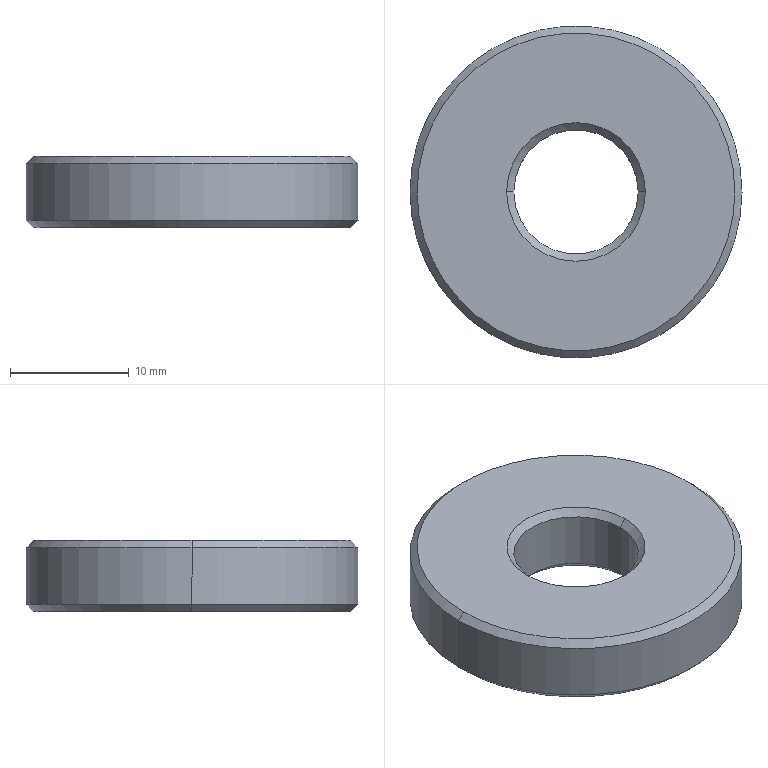Part | SolidWorks | features BaseBody 1 | 1 solid | 38 faces | box 28 x 28 x 6 mm | volume 3096 mm3 | cone 24 | cylinder 12 | plane 2 | commonest cylinder face diameters 2.5 x8 10.5 x2 28 x2
STEP:
#1=CARTESIAN_POINT('',(-5.25,0.,5.4));
#2=VERTEX_POINT('',#1);
#3=CARTESIAN_POINT('',(5.25,0.,5.4));
#4=VERTEX_POINT('',#3);
#5=CARTESIAN_POINT('',(0.,0.,5.4));
#6=DIRECTION('',(0.,0.,1.));
#7=DIRECTION('',(1.,0.,0.));
#8=AXIS2_PLACEMENT_3D('',#5,#6,#7);
#9=CIRCLE('',#8,5.25);
#10=EDGE_CURVE('',#2,#4,#9,.T.);
#11=ORIENTED_EDGE('',*,*,#10,.F.);
#12=CARTESIAN_POINT('',(-5.85,0.,6.));
#13=VERTEX_POINT('',#12);
#14=CARTESIAN_POINT('',(-5.85,0.,6.));
#15=DIRECTION('',(-0.7071,0.,0.7071));
#16=VECTOR('',#15,1000.);
#17=LINE('',#14,#16);
#18=EDGE_CURVE('',#2,#13,#17,.T.);
#19=ORIENTED_EDGE('',*,*,#18,.T.);
#20=CARTESIAN_POINT('',(5.85,0.,6.));
#21=VERTEX_POINT('',#20);
#22=CARTESIAN_POINT('',(0.,0.,6.));
#23=DIRECTION('',(0.,0.,-1.));
#24=DIRECTION('',(1.,0.,0.));
#25=AXIS2_PLACEMENT_3D('',#22,#23,#24);
#26=CIRCLE('',#25,5.85);
#27=EDGE_CURVE('',#21,#13,#26,.T.);
#28=ORIENTED_EDGE('',*,*,#27,.F.);
#29=CARTESIAN_POINT('',(5.85,0.,6.));
#30=DIRECTION('',(0.7071,0.,0.7071));
#31=VECTOR('',#30,1000.);
#32=LINE('',#29,#31);
#33=EDGE_CURVE('',#4,#21,#32,.T.);
#34=ORIENTED_EDGE('',*,*,#33,.F.);
#35=EDGE_LOOP('',(#11,#19,#28,#34));
#36=FACE_OUTER_BOUND('',#35,.T.);
#37=CARTESIAN_POINT('',(0.,0.,6.));
#38=DIRECTION('',(0.,0.,1.));
#39=DIRECTION('',(1.,0.,0.));
#40=AXIS2_PLACEMENT_3D('',#37,#38,#39);
#41=CONICAL_SURFACE('',#40,5.85,0.7854);
#42=ADVANCED_FACE('',(#36),#41,.F.);
#43=CARTESIAN_POINT('',(13.4,0.,6.));
#44=VERTEX_POINT('',#43);
#45=CARTESIAN_POINT('',(-13.4,0.,6.));
#46=VERTEX_POINT('',#45);
#47=CARTESIAN_POINT('',(0.,0.,6.));
#48=DIRECTION('',(0.,0.,1.));
#49=DIRECTION('',(-1.,0.,0.));
#50=AXIS2_PLACEMENT_3D('',#47,#48,#49);
#51=CIRCLE('',#50,13.4);
#52=EDGE_CURVE('',#44,#46,#51,.T.);
#53=ORIENTED_EDGE('',*,*,#52,.F.);
#54=CARTESIAN_POINT('',(14.,0.,5.4));
#55=VERTEX_POINT('',#54);
#56=CARTESIAN_POINT('',(14.,0.,5.4));
#57=DIRECTION('',(0.7071,0.,-0.7071));
#58=VECTOR('',#57,1000.);
#59=LINE('',#56,#58);
#60=EDGE_CURVE('',#44,#55,#59,.T.);
#61=ORIENTED_EDGE('',*,*,#60,.T.);
#62=CARTESIAN_POINT('',(-14.,0.,5.4));
#63=VERTEX_POINT('',#62);
#64=CARTESIAN_POINT('',(0.,0.,5.4));
#65=DIRECTION('',(0.,0.,1.));
#66=DIRECTION('',(-1.,0.,0.));
#67=AXIS2_PLACEMENT_3D('',#64,#65,#66);
#68=CIRCLE('',#67,14.);
#69=EDGE_CURVE('',#55,#63,#68,.T.);
#70=ORIENTED_EDGE('',*,*,#69,.T.);
#71=CARTESIAN_POINT('',(-14.,0.,5.4));
#72=DIRECTION('',(-0.7071,0.,-0.7071));
#73=VECTOR('',#72,1000.);
#74=LINE('',#71,#73);
#75=EDGE_CURVE('',#46,#63,#74,.T.);
#76=ORIENTED_EDGE('',*,*,#75,.F.);
#77=EDGE_LOOP('',(#53,#61,#70,#76));
#78=FACE_OUTER_BOUND('',#77,.T.);
#79=CARTESIAN_POINT('',(0.,0.,5.4));
#80=DIRECTION('',(0.,0.,-1.));
#81=DIRECTION('',(-1.,0.,0.));
#82=AXIS2_PLACEMENT_3D('',#79,#80,#81);
#83=CONICAL_SURFACE('',#82,14.,0.7854);
#84=ADVANCED_FACE('',(#78),#83,.T.);
#85=ORIENTED_EDGE('',*,*,#10,.T.);
#86=CARTESIAN_POINT('',(5.25,0.,0.6));
#87=VERTEX_POINT('',#86);
#88=CARTESIAN_POINT('',(5.25,0.,6.));
#89=DIRECTION('',(0.,0.,-1.));
#90=VECTOR('',#89,1000.);
#91=LINE('',#88,#90);
#92=EDGE_CURVE('',#4,#87,#91,.T.);
#93=ORIENTED_EDGE('',*,*,#92,.T.);
#94=CARTESIAN_POINT('',(-5.25,0.,0.6));
#95=VERTEX_POINT('',#94);
#96=CARTESIAN_POINT('',(0.,0.,0.6));
#97=DIRECTION('',(0.,0.,1.));
#98=DIRECTION('',(-1.,0.,0.));
#99=AXIS2_PLACEMENT_3D('',#96,#97,#98);
#100=CIRCLE('',#99,5.25);
#101=EDGE_CURVE('',#95,#87,#100,.T.);
#102=ORIENTED_EDGE('',*,*,#101,.F.);
#103=CARTESIAN_POINT('',(-5.25,0.,6.));
#104=DIRECTION('',(0.,0.,-1.));
#105=VECTOR('',#104,1000.);
#106=LINE('',#103,#105);
#107=EDGE_CURVE('',#2,#95,#106,.T.);
#108=ORIENTED_EDGE('',*,*,#107,.F.);
#109=EDGE_LOOP('',(#85,#93,#102,#108));
#110=FACE_OUTER_BOUND('',#109,.T.);
#111=CARTESIAN_POINT('',(0.,0.,6.));
#112=DIRECTION('',(0.,0.,-1.));
#113=DIRECTION('',(-1.,0.,0.));
#114=AXIS2_PLACEMENT_3D('',#111,#112,#113);
#115=CYLINDRICAL_SURFACE('',#114,5.25);
#116=ADVANCED_FACE('',(#110),#115,.F.);
#117=ORIENTED_EDGE('',*,*,#69,.F.);
#118=CARTESIAN_POINT('',(14.,0.,0.6));
#119=VERTEX_POINT('',#118);
#120=CARTESIAN_POINT('',(14.,0.,6.));
#121=DIRECTION('',(0.,0.,-1.));
#122=VECTOR('',#121,1000.);
#123=LINE('',#120,#122);
#124=EDGE_CURVE('',#55,#119,#123,.T.);
#125=ORIENTED_EDGE('',*,*,#124,.T.);
#126=CARTESIAN_POINT('',(-14.,0.,0.6));
#127=VERTEX_POINT('',#126);
#128=CARTESIAN_POINT('',(0.,0.,0.6));
#129=DIRECTION('',(0.,0.,1.));
#130=DIRECTION('',(-1.,0.,0.));
#131=AXIS2_PLACEMENT_3D('',#128,#129,#130);
#132=CIRCLE('',#131,14.);
#133=EDGE_CURVE('',#119,#127,#132,.T.);
#134=ORIENTED_EDGE('',*,*,#133,.T.);
#135=CARTESIAN_POINT('',(-14.,0.,6.));
#136=DIRECTION('',(0.,0.,-1.));
#137=VECTOR('',#136,1000.);
#138=LINE('',#135,#137);
#139=EDGE_CURVE('',#63,#127,#138,.T.);
#140=ORIENTED_EDGE('',*,*,#139,.F.);
#141=EDGE_LOOP('',(#117,#125,#134,#140));
#142=FACE_OUTER_BOUND('',#141,.T.);
#143=CARTESIAN_POINT('',(0.,0.,6.));
#144=DIRECTION('',(0.,0.,-1.));
#145=DIRECTION('',(-1.,0.,0.));
#146=AXIS2_PLACEMENT_3D('',#143,#144,#145);
#147=CYLINDRICAL_SURFACE('',#146,14.);
#148=ADVANCED_FACE('',(#142),#147,.T.);
#149=ORIENTED_EDGE('',*,*,#101,.T.);
#150=CARTESIAN_POINT('',(5.85,0.,0.));
#151=VERTEX_POINT('',#150);
#152=CARTESIAN_POINT('',(5.85,0.,0.));
#153=DIRECTION('',(0.7071,0.,-0.7071));
#154=VECTOR('',#153,1000.);
#155=LINE('',#152,#154);
#156=EDGE_CURVE('',#87,#151,#155,.T.);
#157=ORIENTED_EDGE('',*,*,#156,.T.);
#158=CARTESIAN_POINT('',(-5.85,0.,0.));
#159=VERTEX_POINT('',#158);
#160=CARTESIAN_POINT('',(0.,0.,0.));
#161=DIRECTION('',(0.,0.,1.));
#162=DIRECTION('',(-1.,0.,0.));
#163=AXIS2_PLACEMENT_3D('',#160,#161,#162);
#164=CIRCLE('',#163,5.85);
#165=EDGE_CURVE('',#159,#151,#164,.T.);
#166=ORIENTED_EDGE('',*,*,#165,.F.);
#167=CARTESIAN_POINT('',(-5.85,0.,0.));
#168=DIRECTION('',(-0.7071,0.,-0.7071));
#169=VECTOR('',#168,1000.);
#170=LINE('',#167,#169);
#171=EDGE_CURVE('',#95,#159,#170,.T.);
#172=ORIENTED_EDGE('',*,*,#171,.F.);
#173=EDGE_LOOP('',(#149,#157,#166,#172));
#174=FACE_OUTER_BOUND('',#173,.T.);
#175=CARTESIAN_POINT('',(0.,0.,0.));
#176=DIRECTION('',(0.,0.,-1.));
#177=DIRECTION('',(-1.,0.,0.));
#178=AXIS2_PLACEMENT_3D('',#175,#176,#177);
#179=CONICAL_SURFACE('',#178,5.85,0.7854);
#180=ADVANCED_FACE('',(#174),#179,.F.);
#181=CARTESIAN_POINT('',(13.4,0.,0.));
#182=VERTEX_POINT('',#181);
#183=CARTESIAN_POINT('',(-13.4,0.,0.));
#184=VERTEX_POINT('',#183);
#185=CARTESIAN_POINT('',(0.,0.,0.));
#186=DIRECTION('',(0.,0.,1.));
#187=DIRECTION('',(1.,0.,0.));
#188=AXIS2_PLACEMENT_3D('',#185,#186,#187);
#189=CIRCLE('',#188,13.4);
#190=EDGE_CURVE('',#182,#184,#189,.T.);
#191=ORIENTED_EDGE('',*,*,#190,.T.);
#192=CARTESIAN_POINT('',(-14.,0.,0.6));
#193=DIRECTION('',(-0.7071,0.,0.7071));
#194=VECTOR('',#193,1000.);
#195=LINE('',#192,#194);
#196=EDGE_CURVE('',#184,#127,#195,.T.);
#197=ORIENTED_EDGE('',*,*,#196,.T.);
#198=ORIENTED_EDGE('',*,*,#133,.F.);
#199=CARTESIAN_POINT('',(14.,0.,0.6));
#200=DIRECTION('',(0.7071,0.,0.7071));
#201=VECTOR('',#200,1000.);
#202=LINE('',#199,#201);
#203=EDGE_CURVE('',#182,#119,#202,.T.);
#204=ORIENTED_EDGE('',*,*,#203,.F.);
#205=EDGE_LOOP('',(#191,#197,#198,#204));
#206=FACE_OUTER_BOUND('',#205,.T.);
#207=CARTESIAN_POINT('',(0.,0.,0.6));
#208=DIRECTION('',(0.,0.,1.));
#209=DIRECTION('',(1.,0.,0.));
#210=AXIS2_PLACEMENT_3D('',#207,#208,#209);
#211=CONICAL_SURFACE('',#210,14.,0.7854);
#212=ADVANCED_FACE('',(#206),#211,.T.);
#213=CARTESIAN_POINT('',(1.25,9.5,0.4));
#214=VERTEX_POINT('',#213);
#215=CARTESIAN_POINT('',(-1.25,9.5,0.4));
#216=VERTEX_POINT('',#215);
#217=CARTESIAN_POINT('',(0.,9.5,0.4));
#218=DIRECTION('',(0.,0.,-1.));
#219=DIRECTION('',(1.,0.,0.));
#220=AXIS2_PLACEMENT_3D('',#217,#218,#219);
#221=CIRCLE('',#220,1.25);
#222=EDGE_CURVE('',#214,#216,#221,.T.);
#223=ORIENTED_EDGE('',*,*,#222,.F.);
#224=CARTESIAN_POINT('',(1.65,9.5,0.));
#225=VERTEX_POINT('',#224);
#226=CARTESIAN_POINT('',(1.65,9.5,0.));
#227=DIRECTION('',(0.7071,0.,-0.7071));
#228=VECTOR('',#227,1000.);
#229=LINE('',#226,#228);
#230=EDGE_CURVE('',#214,#225,#229,.T.);
#231=ORIENTED_EDGE('',*,*,#230,.T.);
#232=CARTESIAN_POINT('',(-1.65,9.5,0.));
#233=VERTEX_POINT('',#232);
#234=CARTESIAN_POINT('',(0.,9.5,0.));
#235=DIRECTION('',(0.,0.,-1.));
#236=DIRECTION('',(-1.,0.,0.));
#237=AXIS2_PLACEMENT_3D('',#234,#235,#236);
#238=CIRCLE('',#237,1.65);
#239=EDGE_CURVE('',#225,#233,#238,.T.);
#240=ORIENTED_EDGE('',*,*,#239,.T.);
#241=CARTESIAN_POINT('',(-1.65,9.5,0.));
#242=DIRECTION('',(-0.7071,0.,-0.7071));
#243=VECTOR('',#242,1000.);
#244=LINE('',#241,#243);
#245=EDGE_CURVE('',#216,#233,#244,.T.);
#246=ORIENTED_EDGE('',*,*,#245,.F.);
#247=EDGE_LOOP('',(#223,#231,#240,#246));
#248=FACE_OUTER_BOUND('',#247,.T.);
#249=CARTESIAN_POINT('',(0.,9.5,0.));
#250=DIRECTION('',(0.,0.,-1.));
#251=DIRECTION('',(-1.,0.,0.));
#252=AXIS2_PLACEMENT_3D('',#249,#250,#251);
#253=CONICAL_SURFACE('',#252,1.65,0.7854);
#254=ADVANCED_FACE('',(#248),#253,.F.);
#255=CARTESIAN_POINT('',(10.75,0.,0.4));
#256=VERTEX_POINT('',#255);
#257=CARTESIAN_POINT('',(8.25,0.,0.4));
#258=VERTEX_POINT('',#257);
#259=CARTESIAN_POINT('',(9.5,0.,0.4));
#260=DIRECTION('',(0.,0.,-1.));
#261=DIRECTION('',(1.,0.,0.));
#262=AXIS2_PLACEMENT_3D('',#259,#260,#261);
#263=CIRCLE('',#262,1.25);
#264=EDGE_CURVE('',#256,#258,#263,.T.);
#265=ORIENTED_EDGE('',*,*,#264,.F.);
#266=CARTESIAN_POINT('',(11.15,0.,0.));
#267=VERTEX_POINT('',#266);
#268=CARTESIAN_POINT('',(11.15,0.,0.));
#269=DIRECTION('',(0.7071,0.,-0.7071));
#270=VECTOR('',#269,1000.);
#271=LINE('',#268,#270);
#272=EDGE_CURVE('',#256,#267,#271,.T.);
#273=ORIENTED_EDGE('',*,*,#272,.T.);
#274=CARTESIAN_POINT('',(7.85,0.,0.));
#275=VERTEX_POINT('',#274);
#276=CARTESIAN_POINT('',(9.5,0.,0.));
#277=DIRECTION('',(0.,0.,-1.));
#278=DIRECTION('',(-1.,0.,0.));
#279=AXIS2_PLACEMENT_3D('',#276,#277,#278);
#280=CIRCLE('',#279,1.65);
#281=EDGE_CURVE('',#267,#275,#280,.T.);
#282=ORIENTED_EDGE('',*,*,#281,.T.);
#283=CARTESIAN_POINT('',(7.85,0.,0.));
#284=DIRECTION('',(-0.7071,0.,-0.7071));
#285=VECTOR('',#284,1000.);
#286=LINE('',#283,#285);
#287=EDGE_CURVE('',#258,#275,#286,.T.);
#288=ORIENTED_EDGE('',*,*,#287,.F.);
#289=EDGE_LOOP('',(#265,#273,#282,#288));
#290=FACE_OUTER_BOUND('',#289,.T.);
#291=CARTESIAN_POINT('',(9.5,0.,0.));
#292=DIRECTION('',(0.,0.,-1.));
#293=DIRECTION('',(-1.,0.,0.));
#294=AXIS2_PLACEMENT_3D('',#291,#292,#293);
#295=CONICAL_SURFACE('',#294,1.65,0.7854);
#296=ADVANCED_FACE('',(#290),#295,.F.);
#297=CARTESIAN_POINT('',(1.25,-9.5,0.4));
#298=VERTEX_POINT('',#297);
#299=CARTESIAN_POINT('',(-1.25,-9.5,0.4));
#300=VERTEX_POINT('',#299);
#301=CARTESIAN_POINT('',(0.,-9.5,0.4));
#302=DIRECTION('',(0.,0.,-1.));
#303=DIRECTION('',(1.,0.,0.));
#304=AXIS2_PLACEMENT_3D('',#301,#302,#303);
#305=CIRCLE('',#304,1.25);
#306=EDGE_CURVE('',#298,#300,#305,.T.);
#307=ORIENTED_EDGE('',*,*,#306,.F.);
#308=CARTESIAN_POINT('',(1.65,-9.5,0.));
#309=VERTEX_POINT('',#308);
#310=CARTESIAN_POINT('',(1.65,-9.5,0.));
#311=DIRECTION('',(0.7071,0.,-0.7071));
#312=VECTOR('',#311,1000.);
#313=LINE('',#310,#312);
#314=EDGE_CURVE('',#298,#309,#313,.T.);
#315=ORIENTED_EDGE('',*,*,#314,.T.);
#316=CARTESIAN_POINT('',(-1.65,-9.5,0.));
#317=VERTEX_POINT('',#316);
#318=CARTESIAN_POINT('',(0.,-9.5,0.));
#319=DIRECTION('',(0.,0.,-1.));
#320=DIRECTION('',(-1.,0.,0.));
#321=AXIS2_PLACEMENT_3D('',#318,#319,#320);
#322=CIRCLE('',#321,1.65);
#323=EDGE_CURVE('',#309,#317,#322,.T.);
#324=ORIENTED_EDGE('',*,*,#323,.T.);
#325=CARTESIAN_POINT('',(-1.65,-9.5,0.));
#326=DIRECTION('',(-0.7071,0.,-0.7071));
#327=VECTOR('',#326,1000.);
#328=LINE('',#325,#327);
#329=EDGE_CURVE('',#300,#317,#328,.T.);
#330=ORIENTED_EDGE('',*,*,#329,.F.);
#331=EDGE_LOOP('',(#307,#315,#324,#330));
#332=FACE_OUTER_BOUND('',#331,.T.);
#333=CARTESIAN_POINT('',(0.,-9.5,0.));
#334=DIRECTION('',(0.,0.,-1.));
#335=DIRECTION('',(-1.,0.,0.));
#336=AXIS2_PLACEMENT_3D('',#333,#334,#335);
#337=CONICAL_SURFACE('',#336,1.65,0.7854);
#338=ADVANCED_FACE('',(#332),#337,.F.);
#339=CARTESIAN_POINT('',(-8.25,0.,0.4));
#340=VERTEX_POINT('',#339);
#341=CARTESIAN_POINT('',(-10.75,0.,0.4));
#342=VERTEX_POINT('',#341);
#343=CARTESIAN_POINT('',(-9.5,0.,0.4));
#344=DIRECTION('',(0.,0.,-1.));
#345=DIRECTION('',(1.,0.,0.));
#346=AXIS2_PLACEMENT_3D('',#343,#344,#345);
#347=CIRCLE('',#346,1.25);
#348=EDGE_CURVE('',#340,#342,#347,.T.);
#349=ORIENTED_EDGE('',*,*,#348,.F.);
#350=CARTESIAN_POINT('',(-7.85,0.,0.));
#351=VERTEX_POINT('',#350);
#352=CARTESIAN_POINT('',(-7.85,0.,0.));
#353=DIRECTION('',(0.7071,0.,-0.7071));
#354=VECTOR('',#353,1000.);
#355=LINE('',#352,#354);
#356=EDGE_CURVE('',#340,#351,#355,.T.);
#357=ORIENTED_EDGE('',*,*,#356,.T.);
#358=CARTESIAN_POINT('',(-11.15,0.,0.));
#359=VERTEX_POINT('',#358);
#360=CARTESIAN_POINT('',(-9.5,0.,0.));
#361=DIRECTION('',(0.,0.,-1.));
#362=DIRECTION('',(-1.,0.,0.));
#363=AXIS2_PLACEMENT_3D('',#360,#361,#362);
#364=CIRCLE('',#363,1.65);
#365=EDGE_CURVE('',#351,#359,#364,.T.);
#366=ORIENTED_EDGE('',*,*,#365,.T.);
#367=CARTESIAN_POINT('',(-11.15,0.,0.));
#368=DIRECTION('',(-0.7071,0.,-0.7071));
#369=VECTOR('',#368,1000.);
#370=LINE('',#367,#369);
#371=EDGE_CURVE('',#342,#359,#370,.T.);
#372=ORIENTED_EDGE('',*,*,#371,.F.);
#373=EDGE_LOOP('',(#349,#357,#366,#372));
#374=FACE_OUTER_BOUND('',#373,.T.);
#375=CARTESIAN_POINT('',(-9.5,0.,0.));
#376=DIRECTION('',(0.,0.,-1.));
#377=DIRECTION('',(-1.,0.,0.));
#378=AXIS2_PLACEMENT_3D('',#375,#376,#377);
#379=CONICAL_SURFACE('',#378,1.65,0.7854);
#380=ADVANCED_FACE('',(#374),#379,.F.);
#381=ORIENTED_EDGE('',*,*,#222,.T.);
#382=CARTESIAN_POINT('',(-1.25,9.5,1.25));
#383=VERTEX_POINT('',#382);
#384=CARTESIAN_POINT('',(-1.25,9.5,2.5));
#385=DIRECTION('',(0.,0.,1.));
#386=VECTOR('',#385,1000.);
#387=LINE('',#384,#386);
#388=EDGE_CURVE('',#216,#383,#387,.T.);
#389=ORIENTED_EDGE('',*,*,#388,.T.);
#390=CARTESIAN_POINT('',(1.25,9.5,1.25));
#391=VERTEX_POINT('',#390);
#392=CARTESIAN_POINT('',(0.,9.5,1.25));
#393=DIRECTION('',(0.,0.,-1.));
#394=DIRECTION('',(1.,0.,0.));
#395=AXIS2_PLACEMENT_3D('',#392,#393,#394);
#396=CIRCLE('',#395,1.25);
#397=EDGE_CURVE('',#391,#383,#396,.T.);
#398=ORIENTED_EDGE('',*,*,#397,.F.);
#399=CARTESIAN_POINT('',(1.25,9.5,2.5));
#400=DIRECTION('',(0.,0.,1.));
#401=VECTOR('',#400,1000.);
#402=LINE('',#399,#401);
#403=EDGE_CURVE('',#214,#391,#402,.T.);
#404=ORIENTED_EDGE('',*,*,#403,.F.);
#405=EDGE_LOOP('',(#381,#389,#398,#404));
#406=FACE_OUTER_BOUND('',#405,.T.);
#407=CARTESIAN_POINT('',(0.,9.5,2.5));
#408=DIRECTION('',(0.,0.,1.));
#409=DIRECTION('',(1.,0.,0.));
#410=AXIS2_PLACEMENT_3D('',#407,#408,#409);
#411=CYLINDRICAL_SURFACE('',#410,1.25);
#412=ADVANCED_FACE('',(#406),#411,.F.);
#413=ORIENTED_EDGE('',*,*,#264,.T.);
#414=CARTESIAN_POINT('',(8.25,0.,1.25));
#415=VERTEX_POINT('',#414);
#416=CARTESIAN_POINT('',(8.25,0.,2.5));
#417=DIRECTION('',(0.,0.,1.));
#418=VECTOR('',#417,1000.);
#419=LINE('',#416,#418);
#420=EDGE_CURVE('',#258,#415,#419,.T.);
#421=ORIENTED_EDGE('',*,*,#420,.T.);
#422=CARTESIAN_POINT('',(10.75,0.,1.25));
#423=VERTEX_POINT('',#422);
#424=CARTESIAN_POINT('',(9.5,0.,1.25));
#425=DIRECTION('',(0.,0.,-1.));
#426=DIRECTION('',(1.,0.,0.));
#427=AXIS2_PLACEMENT_3D('',#424,#425,#426);
#428=CIRCLE('',#427,1.25);
#429=EDGE_CURVE('',#423,#415,#428,.T.);
#430=ORIENTED_EDGE('',*,*,#429,.F.);
#431=CARTESIAN_POINT('',(10.75,0.,2.5));
#432=DIRECTION('',(0.,0.,1.));
#433=VECTOR('',#432,1000.);
#434=LINE('',#431,#433);
#435=EDGE_CURVE('',#256,#423,#434,.T.);
#436=ORIENTED_EDGE('',*,*,#435,.F.);
#437=EDGE_LOOP('',(#413,#421,#430,#436));
#438=FACE_OUTER_BOUND('',#437,.T.);
#439=CARTESIAN_POINT('',(9.5,0.,2.5));
#440=DIRECTION('',(0.,0.,1.));
#441=DIRECTION('',(1.,0.,0.));
#442=AXIS2_PLACEMENT_3D('',#439,#440,#441);
#443=CYLINDRICAL_SURFACE('',#442,1.25);
#444=ADVANCED_FACE('',(#438),#443,.F.);
#445=ORIENTED_EDGE('',*,*,#306,.T.);
#446=CARTESIAN_POINT('',(-1.25,-9.5,1.25));
#447=VERTEX_POINT('',#446);
#448=CARTESIAN_POINT('',(-1.25,-9.5,2.5));
#449=DIRECTION('',(0.,0.,1.));
#450=VECTOR('',#449,1000.);
#451=LINE('',#448,#450);
#452=EDGE_CURVE('',#300,#447,#451,.T.);
#453=ORIENTED_EDGE('',*,*,#452,.T.);
#454=CARTESIAN_POINT('',(1.25,-9.5,1.25));
#455=VERTEX_POINT('',#454);
#456=CARTESIAN_POINT('',(0.,-9.5,1.25));
#457=DIRECTION('',(0.,0.,-1.));
#458=DIRECTION('',(1.,0.,0.));
#459=AXIS2_PLACEMENT_3D('',#456,#457,#458);
#460=CIRCLE('',#459,1.25);
#461=EDGE_CURVE('',#455,#447,#460,.T.);
#462=ORIENTED_EDGE('',*,*,#461,.F.);
#463=CARTESIAN_POINT('',(1.25,-9.5,2.5));
#464=DIRECTION('',(0.,0.,1.));
#465=VECTOR('',#464,1000.);
#466=LINE('',#463,#465);
#467=EDGE_CURVE('',#298,#455,#466,.T.);
#468=ORIENTED_EDGE('',*,*,#467,.F.);
#469=EDGE_LOOP('',(#445,#453,#462,#468));
#470=FACE_OUTER_BOUND('',#469,.T.);
#471=CARTESIAN_POINT('',(0.,-9.5,2.5));
#472=DIRECTION('',(0.,0.,1.));
#473=DIRECTION('',(1.,0.,0.));
#474=AXIS2_PLACEMENT_3D('',#471,#472,#473);
#475=CYLINDRICAL_SURFACE('',#474,1.25);
#476=ADVANCED_FACE('',(#470),#475,.F.);
#477=ORIENTED_EDGE('',*,*,#348,.T.);
#478=CARTESIAN_POINT('',(-10.75,0.,1.25));
#479=VERTEX_POINT('',#478);
#480=CARTESIAN_POINT('',(-10.75,0.,2.5));
#481=DIRECTION('',(0.,0.,1.));
#482=VECTOR('',#481,1000.);
#483=LINE('',#480,#482);
#484=EDGE_CURVE('',#342,#479,#483,.T.);
#485=ORIENTED_EDGE('',*,*,#484,.T.);
#486=CARTESIAN_POINT('',(-8.25,0.,1.25));
#487=VERTEX_POINT('',#486);
#488=CARTESIAN_POINT('',(-9.5,0.,1.25));
#489=DIRECTION('',(0.,0.,-1.));
#490=DIRECTION('',(1.,0.,0.));
#491=AXIS2_PLACEMENT_3D('',#488,#489,#490);
#492=CIRCLE('',#491,1.25);
#493=EDGE_CURVE('',#487,#479,#492,.T.);
#494=ORIENTED_EDGE('',*,*,#493,.F.);
#495=CARTESIAN_POINT('',(-8.25,0.,2.5));
#496=DIRECTION('',(0.,0.,1.));
#497=VECTOR('',#496,1000.);
#498=LINE('',#495,#497);
#499=EDGE_CURVE('',#340,#487,#498,.T.);
#500=ORIENTED_EDGE('',*,*,#499,.F.);
#501=EDGE_LOOP('',(#477,#485,#494,#500));
#502=FACE_OUTER_BOUND('',#501,.T.);
#503=CARTESIAN_POINT('',(-9.5,0.,2.5));
#504=DIRECTION('',(0.,0.,1.));
#505=DIRECTION('',(1.,0.,0.));
#506=AXIS2_PLACEMENT_3D('',#503,#504,#505);
#507=CYLINDRICAL_SURFACE('',#506,1.25);
#508=ADVANCED_FACE('',(#502),#507,.F.);
#509=CARTESIAN_POINT('',(0.,9.5,2.5));
#510=VERTEX_POINT('',#509);
#511=CARTESIAN_POINT('',(-1.25,9.5,1.25));
#512=DIRECTION('',(-0.7071,0.,-0.7071));
#513=VECTOR('',#512,1000.);
#514=LINE('',#511,#513);
#515=EDGE_CURVE('',#510,#383,#514,.T.);
#516=ORIENTED_EDGE('',*,*,#515,.F.);
#517=CARTESIAN_POINT('',(1.25,9.5,1.25));
#518=DIRECTION('',(0.7071,0.,-0.7071));
#519=VECTOR('',#518,1000.);
#520=LINE('',#517,#519);
#521=EDGE_CURVE('',#510,#391,#520,.T.);
#522=ORIENTED_EDGE('',*,*,#521,.T.);
#523=ORIENTED_EDGE('',*,*,#397,.T.);
#524=EDGE_LOOP('',(#516,#522,#523));
#525=FACE_OUTER_BOUND('',#524,.T.);
#526=CARTESIAN_POINT('',(0.,9.5,1.25));
#527=DIRECTION('',(0.,0.,-1.));
#528=DIRECTION('',(-1.,0.,0.));
#529=AXIS2_PLACEMENT_3D('',#526,#527,#528);
#530=CONICAL_SURFACE('',#529,1.25,0.7854);
#531=ADVANCED_FACE('',(#525),#530,.F.);
#532=CARTESIAN_POINT('',(9.5,0.,2.5));
#533=VERTEX_POINT('',#532);
#534=CARTESIAN_POINT('',(8.25,0.,1.25));
#535=DIRECTION('',(-0.7071,0.,-0.7071));
#536=VECTOR('',#535,1000.);
#537=LINE('',#534,#536);
#538=EDGE_CURVE('',#533,#415,#537,.T.);
#539=ORIENTED_EDGE('',*,*,#538,.F.);
#540=CARTESIAN_POINT('',(10.75,0.,1.25));
#541=DIRECTION('',(0.7071,0.,-0.7071));
#542=VECTOR('',#541,1000.);
#543=LINE('',#540,#542);
#544=EDGE_CURVE('',#533,#423,#543,.T.);
#545=ORIENTED_EDGE('',*,*,#544,.T.);
#546=ORIENTED_EDGE('',*,*,#429,.T.);
#547=EDGE_LOOP('',(#539,#545,#546));
#548=FACE_OUTER_BOUND('',#547,.T.);
#549=CARTESIAN_POINT('',(9.5,0.,1.25));
#550=DIRECTION('',(0.,0.,-1.));
#551=DIRECTION('',(-1.,0.,0.));
#552=AXIS2_PLACEMENT_3D('',#549,#550,#551);
#553=CONICAL_SURFACE('',#552,1.25,0.7854);
#554=ADVANCED_FACE('',(#548),#553,.F.);
#555=CARTESIAN_POINT('',(0.,-9.5,2.5));
#556=VERTEX_POINT('',#555);
#557=CARTESIAN_POINT('',(-1.25,-9.5,1.25));
#558=DIRECTION('',(-0.7071,0.,-0.7071));
#559=VECTOR('',#558,1000.);
#560=LINE('',#557,#559);
#561=EDGE_CURVE('',#556,#447,#560,.T.);
#562=ORIENTED_EDGE('',*,*,#561,.F.);
#563=CARTESIAN_POINT('',(1.25,-9.5,1.25));
#564=DIRECTION('',(0.7071,0.,-0.7071));
#565=VECTOR('',#564,1000.);
#566=LINE('',#563,#565);
#567=EDGE_CURVE('',#556,#455,#566,.T.);
#568=ORIENTED_EDGE('',*,*,#567,.T.);
#569=ORIENTED_EDGE('',*,*,#461,.T.);
#570=EDGE_LOOP('',(#562,#568,#569));
#571=FACE_OUTER_BOUND('',#570,.T.);
#572=CARTESIAN_POINT('',(0.,-9.5,1.25));
#573=DIRECTION('',(0.,0.,-1.));
#574=DIRECTION('',(-1.,0.,0.));
#575=AXIS2_PLACEMENT_3D('',#572,#573,#574);
#576=CONICAL_SURFACE('',#575,1.25,0.7854);
#577=ADVANCED_FACE('',(#571),#576,.F.);
#578=CARTESIAN_POINT('',(-9.5,0.,2.5));
#579=VERTEX_POINT('',#578);
#580=CARTESIAN_POINT('',(-10.75,0.,1.25));
#581=DIRECTION('',(-0.7071,0.,-0.7071));
#582=VECTOR('',#581,1000.);
#583=LINE('',#580,#582);
#584=EDGE_CURVE('',#579,#479,#583,.T.);
#585=ORIENTED_EDGE('',*,*,#584,.F.);
#586=CARTESIAN_POINT('',(-8.25,0.,1.25));
#587=DIRECTION('',(0.7071,0.,-0.7071));
#588=VECTOR('',#587,1000.);
#589=LINE('',#586,#588);
#590=EDGE_CURVE('',#579,#487,#589,.T.);
#591=ORIENTED_EDGE('',*,*,#590,.T.);
#592=ORIENTED_EDGE('',*,*,#493,.T.);
#593=EDGE_LOOP('',(#585,#591,#592));
#594=FACE_OUTER_BOUND('',#593,.T.);
#595=CARTESIAN_POINT('',(-9.5,0.,1.25));
#596=DIRECTION('',(0.,0.,-1.));
#597=DIRECTION('',(-1.,0.,0.));
#598=AXIS2_PLACEMENT_3D('',#595,#596,#597);
#599=CONICAL_SURFACE('',#598,1.25,0.7854);
#600=ADVANCED_FACE('',(#594),#599,.F.);
#601=ORIENTED_EDGE('',*,*,#27,.T.);
#602=CARTESIAN_POINT('',(0.,0.,6.));
#603=DIRECTION('',(0.,0.,-1.));
#604=DIRECTION('',(1.,0.,0.));
#605=AXIS2_PLACEMENT_3D('',#602,#603,#604);
#606=CIRCLE('',#605,5.85);
#607=EDGE_CURVE('',#13,#21,#606,.T.);
#608=ORIENTED_EDGE('',*,*,#607,.T.);
#609=EDGE_LOOP('',(#601,#608));
#610=FACE_BOUND('',#609,.T.);
#611=CARTESIAN_POINT('',(0.,0.,6.));
#612=DIRECTION('',(0.,0.,1.));
#613=DIRECTION('',(-1.,0.,0.));
#614=AXIS2_PLACEMENT_3D('',#611,#612,#613);
#615=CIRCLE('',#614,13.4);
#616=EDGE_CURVE('',#46,#44,#615,.T.);
#617=ORIENTED_EDGE('',*,*,#616,.T.);
#618=ORIENTED_EDGE('',*,*,#52,.T.);
#619=EDGE_LOOP('',(#617,#618));
#620=FACE_OUTER_BOUND('',#619,.T.);
#621=CARTESIAN_POINT('',(0.,0.,6.));
#622=DIRECTION('',(0.,0.,1.));
#623=DIRECTION('',(1.,0.,0.));
#624=AXIS2_PLACEMENT_3D('',#621,#622,#623);
#625=PLANE('',#624);
#626=ADVANCED_FACE('',(#610,#620),#625,.T.);
#627=ORIENTED_EDGE('',*,*,#18,.F.);
#628=CARTESIAN_POINT('',(0.,0.,5.4));
#629=DIRECTION('',(0.,0.,1.));
#630=DIRECTION('',(1.,0.,0.));
#631=AXIS2_PLACEMENT_3D('',#628,#629,#630);
#632=CIRCLE('',#631,5.25);
#633=EDGE_CURVE('',#4,#2,#632,.T.);
#634=ORIENTED_EDGE('',*,*,#633,.F.);
#635=ORIENTED_EDGE('',*,*,#33,.T.);
#636=ORIENTED_EDGE('',*,*,#607,.F.);
#637=EDGE_LOOP('',(#627,#634,#635,#636));
#638=FACE_OUTER_BOUND('',#637,.T.);
#639=CARTESIAN_POINT('',(0.,0.,6.));
#640=DIRECTION('',(0.,0.,1.));
#641=DIRECTION('',(1.,0.,0.));
#642=AXIS2_PLACEMENT_3D('',#639,#640,#641);
#643=CONICAL_SURFACE('',#642,5.85,0.7854);
#644=ADVANCED_FACE('',(#638),#643,.F.);
#645=ORIENTED_EDGE('',*,*,#60,.F.);
#646=ORIENTED_EDGE('',*,*,#616,.F.);
#647=ORIENTED_EDGE('',*,*,#75,.T.);
#648=CARTESIAN_POINT('',(0.,0.,5.4));
#649=DIRECTION('',(0.,0.,1.));
#650=DIRECTION('',(-1.,0.,0.));
#651=AXIS2_PLACEMENT_3D('',#648,#649,#650);
#652=CIRCLE('',#651,14.);
#653=EDGE_CURVE('',#63,#55,#652,.T.);
#654=ORIENTED_EDGE('',*,*,#653,.T.);
#655=EDGE_LOOP('',(#645,#646,#647,#654));
#656=FACE_OUTER_BOUND('',#655,.T.);
#657=CARTESIAN_POINT('',(0.,0.,5.4));
#658=DIRECTION('',(0.,0.,-1.));
#659=DIRECTION('',(-1.,0.,0.));
#660=AXIS2_PLACEMENT_3D('',#657,#658,#659);
#661=CONICAL_SURFACE('',#660,14.,0.7854);
#662=ADVANCED_FACE('',(#656),#661,.T.);
#663=ORIENTED_EDGE('',*,*,#92,.F.);
#664=ORIENTED_EDGE('',*,*,#633,.T.);
#665=ORIENTED_EDGE('',*,*,#107,.T.);
#666=CARTESIAN_POINT('',(0.,0.,0.6));
#667=DIRECTION('',(0.,0.,1.));
#668=DIRECTION('',(-1.,0.,0.));
#669=AXIS2_PLACEMENT_3D('',#666,#667,#668);
#670=CIRCLE('',#669,5.25);
#671=EDGE_CURVE('',#87,#95,#670,.T.);
#672=ORIENTED_EDGE('',*,*,#671,.F.);
#673=EDGE_LOOP('',(#663,#664,#665,#672));
#674=FACE_OUTER_BOUND('',#673,.T.);
#675=CARTESIAN_POINT('',(0.,0.,6.));
#676=DIRECTION('',(0.,0.,-1.));
#677=DIRECTION('',(-1.,0.,0.));
#678=AXIS2_PLACEMENT_3D('',#675,#676,#677);
#679=CYLINDRICAL_SURFACE('',#678,5.25);
#680=ADVANCED_FACE('',(#674),#679,.F.);
#681=ORIENTED_EDGE('',*,*,#124,.F.);
#682=ORIENTED_EDGE('',*,*,#653,.F.);
#683=ORIENTED_EDGE('',*,*,#139,.T.);
#684=CARTESIAN_POINT('',(0.,0.,0.6));
#685=DIRECTION('',(0.,0.,1.));
#686=DIRECTION('',(-1.,0.,0.));
#687=AXIS2_PLACEMENT_3D('',#684,#685,#686);
#688=CIRCLE('',#687,14.);
#689=EDGE_CURVE('',#127,#119,#688,.T.);
#690=ORIENTED_EDGE('',*,*,#689,.T.);
#691=EDGE_LOOP('',(#681,#682,#683,#690));
#692=FACE_OUTER_BOUND('',#691,.T.);
#693=CARTESIAN_POINT('',(0.,0.,6.));
#694=DIRECTION('',(0.,0.,-1.));
#695=DIRECTION('',(-1.,0.,0.));
#696=AXIS2_PLACEMENT_3D('',#693,#694,#695);
#697=CYLINDRICAL_SURFACE('',#696,14.);
#698=ADVANCED_FACE('',(#692),#697,.T.);
#699=ORIENTED_EDGE('',*,*,#156,.F.);
#700=ORIENTED_EDGE('',*,*,#671,.T.);
#701=ORIENTED_EDGE('',*,*,#171,.T.);
#702=CARTESIAN_POINT('',(0.,0.,0.));
#703=DIRECTION('',(0.,0.,1.));
#704=DIRECTION('',(-1.,0.,0.));
#705=AXIS2_PLACEMENT_3D('',#702,#703,#704);
#706=CIRCLE('',#705,5.85);
#707=EDGE_CURVE('',#151,#159,#706,.T.);
#708=ORIENTED_EDGE('',*,*,#707,.F.);
#709=EDGE_LOOP('',(#699,#700,#701,#708));
#710=FACE_OUTER_BOUND('',#709,.T.);
#711=CARTESIAN_POINT('',(0.,0.,0.));
#712=DIRECTION('',(0.,0.,-1.));
#713=DIRECTION('',(-1.,0.,0.));
#714=AXIS2_PLACEMENT_3D('',#711,#712,#713);
#715=CONICAL_SURFACE('',#714,5.85,0.7854);
#716=ADVANCED_FACE('',(#710),#715,.F.);
#717=ORIENTED_EDGE('',*,*,#196,.F.);
#718=CARTESIAN_POINT('',(0.,0.,0.));
#719=DIRECTION('',(0.,0.,1.));
#720=DIRECTION('',(1.,0.,0.));
#721=AXIS2_PLACEMENT_3D('',#718,#719,#720);
#722=CIRCLE('',#721,13.4);
#723=EDGE_CURVE('',#184,#182,#722,.T.);
#724=ORIENTED_EDGE('',*,*,#723,.T.);
#725=ORIENTED_EDGE('',*,*,#203,.T.);
#726=ORIENTED_EDGE('',*,*,#689,.F.);
#727=EDGE_LOOP('',(#717,#724,#725,#726));
#728=FACE_OUTER_BOUND('',#727,.T.);
#729=CARTESIAN_POINT('',(0.,0.,0.6));
#730=DIRECTION('',(0.,0.,1.));
#731=DIRECTION('',(1.,0.,0.));
#732=AXIS2_PLACEMENT_3D('',#729,#730,#731);
#733=CONICAL_SURFACE('',#732,14.,0.7854);
#734=ADVANCED_FACE('',(#728),#733,.T.);
#735=ORIENTED_EDGE('',*,*,#165,.T.);
#736=ORIENTED_EDGE('',*,*,#707,.T.);
#737=EDGE_LOOP('',(#735,#736));
#738=FACE_BOUND('',#737,.T.);
#739=CARTESIAN_POINT('',(0.,9.5,0.));
#740=DIRECTION('',(0.,0.,-1.));
#741=DIRECTION('',(-1.,0.,0.));
#742=AXIS2_PLACEMENT_3D('',#739,#740,#741);
#743=CIRCLE('',#742,1.65);
#744=EDGE_CURVE('',#233,#225,#743,.T.);
#745=ORIENTED_EDGE('',*,*,#744,.F.);
#746=ORIENTED_EDGE('',*,*,#239,.F.);
#747=EDGE_LOOP('',(#745,#746));
#748=FACE_BOUND('',#747,.T.);
#749=CARTESIAN_POINT('',(9.5,0.,0.));
#750=DIRECTION('',(0.,0.,-1.));
#751=DIRECTION('',(-1.,0.,0.));
#752=AXIS2_PLACEMENT_3D('',#749,#750,#751);
#753=CIRCLE('',#752,1.65);
#754=EDGE_CURVE('',#275,#267,#753,.T.);
#755=ORIENTED_EDGE('',*,*,#754,.F.);
#756=ORIENTED_EDGE('',*,*,#281,.F.);
#757=EDGE_LOOP('',(#755,#756));
#758=FACE_BOUND('',#757,.T.);
#759=CARTESIAN_POINT('',(0.,-9.5,0.));
#760=DIRECTION('',(0.,0.,-1.));
#761=DIRECTION('',(-1.,0.,0.));
#762=AXIS2_PLACEMENT_3D('',#759,#760,#761);
#763=CIRCLE('',#762,1.65);
#764=EDGE_CURVE('',#317,#309,#763,.T.);
#765=ORIENTED_EDGE('',*,*,#764,.F.);
#766=ORIENTED_EDGE('',*,*,#323,.F.);
#767=EDGE_LOOP('',(#765,#766));
#768=FACE_BOUND('',#767,.T.);
#769=CARTESIAN_POINT('',(-9.5,0.,0.));
#770=DIRECTION('',(0.,0.,-1.));
#771=DIRECTION('',(-1.,0.,0.));
#772=AXIS2_PLACEMENT_3D('',#769,#770,#771);
#773=CIRCLE('',#772,1.65);
#774=EDGE_CURVE('',#359,#351,#773,.T.);
#775=ORIENTED_EDGE('',*,*,#774,.F.);
#776=ORIENTED_EDGE('',*,*,#365,.F.);
#777=EDGE_LOOP('',(#775,#776));
#778=FACE_BOUND('',#777,.T.);
#779=ORIENTED_EDGE('',*,*,#190,.F.);
#780=ORIENTED_EDGE('',*,*,#723,.F.);
#781=EDGE_LOOP('',(#779,#780));
#782=FACE_OUTER_BOUND('',#781,.T.);
#783=CARTESIAN_POINT('',(0.,0.,0.));
#784=DIRECTION('',(0.,0.,1.));
#785=DIRECTION('',(1.,0.,0.));
#786=AXIS2_PLACEMENT_3D('',#783,#784,#785);
#787=PLANE('',#786);
#788=ADVANCED_FACE('',(#738,#748,#758,#768,#778,#782),#787,.F.);
#789=ORIENTED_EDGE('',*,*,#230,.F.);
#790=CARTESIAN_POINT('',(0.,9.5,0.4));
#791=DIRECTION('',(0.,0.,-1.));
#792=DIRECTION('',(1.,0.,0.));
#793=AXIS2_PLACEMENT_3D('',#790,#791,#792);
#794=CIRCLE('',#793,1.25);
#795=EDGE_CURVE('',#216,#214,#794,.T.);
#796=ORIENTED_EDGE('',*,*,#795,.F.);
#797=ORIENTED_EDGE('',*,*,#245,.T.);
#798=ORIENTED_EDGE('',*,*,#744,.T.);
#799=EDGE_LOOP('',(#789,#796,#797,#798));
#800=FACE_OUTER_BOUND('',#799,.T.);
#801=CARTESIAN_POINT('',(0.,9.5,0.));
#802=DIRECTION('',(0.,0.,-1.));
#803=DIRECTION('',(-1.,0.,0.));
#804=AXIS2_PLACEMENT_3D('',#801,#802,#803);
#805=CONICAL_SURFACE('',#804,1.65,0.7854);
#806=ADVANCED_FACE('',(#800),#805,.F.);
#807=ORIENTED_EDGE('',*,*,#272,.F.);
#808=CARTESIAN_POINT('',(9.5,0.,0.4));
#809=DIRECTION('',(0.,0.,-1.));
#810=DIRECTION('',(1.,0.,0.));
#811=AXIS2_PLACEMENT_3D('',#808,#809,#810);
#812=CIRCLE('',#811,1.25);
#813=EDGE_CURVE('',#258,#256,#812,.T.);
#814=ORIENTED_EDGE('',*,*,#813,.F.);
#815=ORIENTED_EDGE('',*,*,#287,.T.);
#816=ORIENTED_EDGE('',*,*,#754,.T.);
#817=EDGE_LOOP('',(#807,#814,#815,#816));
#818=FACE_OUTER_BOUND('',#817,.T.);
#819=CARTESIAN_POINT('',(9.5,0.,0.));
#820=DIRECTION('',(0.,0.,-1.));
#821=DIRECTION('',(-1.,0.,0.));
#822=AXIS2_PLACEMENT_3D('',#819,#820,#821);
#823=CONICAL_SURFACE('',#822,1.65,0.7854);
#824=ADVANCED_FACE('',(#818),#823,.F.);
#825=ORIENTED_EDGE('',*,*,#314,.F.);
#826=CARTESIAN_POINT('',(0.,-9.5,0.4));
#827=DIRECTION('',(0.,0.,-1.));
#828=DIRECTION('',(1.,0.,0.));
#829=AXIS2_PLACEMENT_3D('',#826,#827,#828);
#830=CIRCLE('',#829,1.25);
#831=EDGE_CURVE('',#300,#298,#830,.T.);
#832=ORIENTED_EDGE('',*,*,#831,.F.);
#833=ORIENTED_EDGE('',*,*,#329,.T.);
#834=ORIENTED_EDGE('',*,*,#764,.T.);
#835=EDGE_LOOP('',(#825,#832,#833,#834));
#836=FACE_OUTER_BOUND('',#835,.T.);
#837=CARTESIAN_POINT('',(0.,-9.5,0.));
#838=DIRECTION('',(0.,0.,-1.));
#839=DIRECTION('',(-1.,0.,0.));
#840=AXIS2_PLACEMENT_3D('',#837,#838,#839);
#841=CONICAL_SURFACE('',#840,1.65,0.7854);
#842=ADVANCED_FACE('',(#836),#841,.F.);
#843=ORIENTED_EDGE('',*,*,#356,.F.);
#844=CARTESIAN_POINT('',(-9.5,0.,0.4));
#845=DIRECTION('',(0.,0.,-1.));
#846=DIRECTION('',(1.,0.,0.));
#847=AXIS2_PLACEMENT_3D('',#844,#845,#846);
#848=CIRCLE('',#847,1.25);
#849=EDGE_CURVE('',#342,#340,#848,.T.);
#850=ORIENTED_EDGE('',*,*,#849,.F.);
#851=ORIENTED_EDGE('',*,*,#371,.T.);
#852=ORIENTED_EDGE('',*,*,#774,.T.);
#853=EDGE_LOOP('',(#843,#850,#851,#852));
#854=FACE_OUTER_BOUND('',#853,.T.);
#855=CARTESIAN_POINT('',(-9.5,0.,0.));
#856=DIRECTION('',(0.,0.,-1.));
#857=DIRECTION('',(-1.,0.,0.));
#858=AXIS2_PLACEMENT_3D('',#855,#856,#857);
#859=CONICAL_SURFACE('',#858,1.65,0.7854);
#860=ADVANCED_FACE('',(#854),#859,.F.);
#861=ORIENTED_EDGE('',*,*,#388,.F.);
#862=ORIENTED_EDGE('',*,*,#795,.T.);
#863=ORIENTED_EDGE('',*,*,#403,.T.);
#864=CARTESIAN_POINT('',(0.,9.5,1.25));
#865=DIRECTION('',(0.,0.,-1.));
#866=DIRECTION('',(1.,0.,0.));
#867=AXIS2_PLACEMENT_3D('',#864,#865,#866);
#868=CIRCLE('',#867,1.25);
#869=EDGE_CURVE('',#383,#391,#868,.T.);
#870=ORIENTED_EDGE('',*,*,#869,.F.);
#871=EDGE_LOOP('',(#861,#862,#863,#870));
#872=FACE_OUTER_BOUND('',#871,.T.);
#873=CARTESIAN_POINT('',(0.,9.5,2.5));
#874=DIRECTION('',(0.,0.,1.));
#875=DIRECTION('',(1.,0.,0.));
#876=AXIS2_PLACEMENT_3D('',#873,#874,#875);
#877=CYLINDRICAL_SURFACE('',#876,1.25);
#878=ADVANCED_FACE('',(#872),#877,.F.);
#879=ORIENTED_EDGE('',*,*,#420,.F.);
#880=ORIENTED_EDGE('',*,*,#813,.T.);
#881=ORIENTED_EDGE('',*,*,#435,.T.);
#882=CARTESIAN_POINT('',(9.5,0.,1.25));
#883=DIRECTION('',(0.,0.,-1.));
#884=DIRECTION('',(1.,0.,0.));
#885=AXIS2_PLACEMENT_3D('',#882,#883,#884);
#886=CIRCLE('',#885,1.25);
#887=EDGE_CURVE('',#415,#423,#886,.T.);
#888=ORIENTED_EDGE('',*,*,#887,.F.);
#889=EDGE_LOOP('',(#879,#880,#881,#888));
#890=FACE_OUTER_BOUND('',#889,.T.);
#891=CARTESIAN_POINT('',(9.5,0.,2.5));
#892=DIRECTION('',(0.,0.,1.));
#893=DIRECTION('',(1.,0.,0.));
#894=AXIS2_PLACEMENT_3D('',#891,#892,#893);
#895=CYLINDRICAL_SURFACE('',#894,1.25);
#896=ADVANCED_FACE('',(#890),#895,.F.);
#897=ORIENTED_EDGE('',*,*,#452,.F.);
#898=ORIENTED_EDGE('',*,*,#831,.T.);
#899=ORIENTED_EDGE('',*,*,#467,.T.);
#900=CARTESIAN_POINT('',(0.,-9.5,1.25));
#901=DIRECTION('',(0.,0.,-1.));
#902=DIRECTION('',(1.,0.,0.));
#903=AXIS2_PLACEMENT_3D('',#900,#901,#902);
#904=CIRCLE('',#903,1.25);
#905=EDGE_CURVE('',#447,#455,#904,.T.);
#906=ORIENTED_EDGE('',*,*,#905,.F.);
#907=EDGE_LOOP('',(#897,#898,#899,#906));
#908=FACE_OUTER_BOUND('',#907,.T.);
#909=CARTESIAN_POINT('',(0.,-9.5,2.5));
#910=DIRECTION('',(0.,0.,1.));
#911=DIRECTION('',(1.,0.,0.));
#912=AXIS2_PLACEMENT_3D('',#909,#910,#911);
#913=CYLINDRICAL_SURFACE('',#912,1.25);
#914=ADVANCED_FACE('',(#908),#913,.F.);
#915=ORIENTED_EDGE('',*,*,#484,.F.);
#916=ORIENTED_EDGE('',*,*,#849,.T.);
#917=ORIENTED_EDGE('',*,*,#499,.T.);
#918=CARTESIAN_POINT('',(-9.5,0.,1.25));
#919=DIRECTION('',(0.,0.,-1.));
#920=DIRECTION('',(1.,0.,0.));
#921=AXIS2_PLACEMENT_3D('',#918,#919,#920);
#922=CIRCLE('',#921,1.25);
#923=EDGE_CURVE('',#479,#487,#922,.T.);
#924=ORIENTED_EDGE('',*,*,#923,.F.);
#925=EDGE_LOOP('',(#915,#916,#917,#924));
#926=FACE_OUTER_BOUND('',#925,.T.);
#927=CARTESIAN_POINT('',(-9.5,0.,2.5));
#928=DIRECTION('',(0.,0.,1.));
#929=DIRECTION('',(1.,0.,0.));
#930=AXIS2_PLACEMENT_3D('',#927,#928,#929);
#931=CYLINDRICAL_SURFACE('',#930,1.25);
#932=ADVANCED_FACE('',(#926),#931,.F.);
#933=ORIENTED_EDGE('',*,*,#521,.F.);
#934=ORIENTED_EDGE('',*,*,#515,.T.);
#935=ORIENTED_EDGE('',*,*,#869,.T.);
#936=EDGE_LOOP('',(#933,#934,#935));
#937=FACE_OUTER_BOUND('',#936,.T.);
#938=CARTESIAN_POINT('',(0.,9.5,1.25));
#939=DIRECTION('',(0.,0.,-1.));
#940=DIRECTION('',(-1.,0.,0.));
#941=AXIS2_PLACEMENT_3D('',#938,#939,#940);
#942=CONICAL_SURFACE('',#941,1.25,0.7854);
#943=ADVANCED_FACE('',(#937),#942,.F.);
#944=ORIENTED_EDGE('',*,*,#544,.F.);
#945=ORIENTED_EDGE('',*,*,#538,.T.);
#946=ORIENTED_EDGE('',*,*,#887,.T.);
#947=EDGE_LOOP('',(#944,#945,#946));
#948=FACE_OUTER_BOUND('',#947,.T.);
#949=CARTESIAN_POINT('',(9.5,0.,1.25));
#950=DIRECTION('',(0.,0.,-1.));
#951=DIRECTION('',(-1.,0.,0.));
#952=AXIS2_PLACEMENT_3D('',#949,#950,#951);
#953=CONICAL_SURFACE('',#952,1.25,0.7854);
#954=ADVANCED_FACE('',(#948),#953,.F.);
#955=ORIENTED_EDGE('',*,*,#567,.F.);
#956=ORIENTED_EDGE('',*,*,#561,.T.);
#957=ORIENTED_EDGE('',*,*,#905,.T.);
#958=EDGE_LOOP('',(#955,#956,#957));
#959=FACE_OUTER_BOUND('',#958,.T.);
#960=CARTESIAN_POINT('',(0.,-9.5,1.25));
#961=DIRECTION('',(0.,0.,-1.));
#962=DIRECTION('',(-1.,0.,0.));
#963=AXIS2_PLACEMENT_3D('',#960,#961,#962);
#964=CONICAL_SURFACE('',#963,1.25,0.7854);
#965=ADVANCED_FACE('',(#959),#964,.F.);
#966=ORIENTED_EDGE('',*,*,#590,.F.);
#967=ORIENTED_EDGE('',*,*,#584,.T.);
#968=ORIENTED_EDGE('',*,*,#923,.T.);
#969=EDGE_LOOP('',(#966,#967,#968));
#970=FACE_OUTER_BOUND('',#969,.T.);
#971=CARTESIAN_POINT('',(-9.5,0.,1.25));
#972=DIRECTION('',(0.,0.,-1.));
#973=DIRECTION('',(-1.,0.,0.));
#974=AXIS2_PLACEMENT_3D('',#971,#972,#973);
#975=CONICAL_SURFACE('',#974,1.25,0.7854);
#976=ADVANCED_FACE('',(#970),#975,.F.);
#977=CLOSED_SHELL('',(#42,#84,#116,#148,#180,#212,#254,#296,#338,#380,#412,#444,#476,#508,#531,#554,#577,#600,#626,#644,#662,#680,#698,#716,#734,#788,#806,#824,#842,#860,#878,#896,#914,#932,#943,#954,#965,#976));
#978=MANIFOLD_SOLID_BREP('',#977);
#979=CARTESIAN_POINT('',(0.,0.,0.));
#980=DIRECTION('',(0.,0.,1.));
#981=DIRECTION('',(1.,0.,0.));
#982=AXIS2_PLACEMENT_3D('',#979,#980,#981);
#983=(LENGTH_UNIT()NAMED_UNIT(*)SI_UNIT(.MILLI.,.METRE.));
#984=UNCERTAINTY_MEASURE_WITH_UNIT(LENGTH_MEASURE(0.00001),#983,'','');
#985=(NAMED_UNIT(*)PLANE_ANGLE_UNIT()SI_UNIT($,.RADIAN.));
#986=(NAMED_UNIT(*)SI_UNIT($,.STERADIAN.)SOLID_ANGLE_UNIT());
#987=(GEOMETRIC_REPRESENTATION_CONTEXT(3)GLOBAL_UNCERTAINTY_ASSIGNED_CONTEXT((#984))GLOBAL_UNIT_ASSIGNED_CONTEXT((#983,#985,#986))REPRESENTATION_CONTEXT('',''));
#988=ADVANCED_BREP_SHAPE_REPRESENTATION('',(#978,#982),#987);